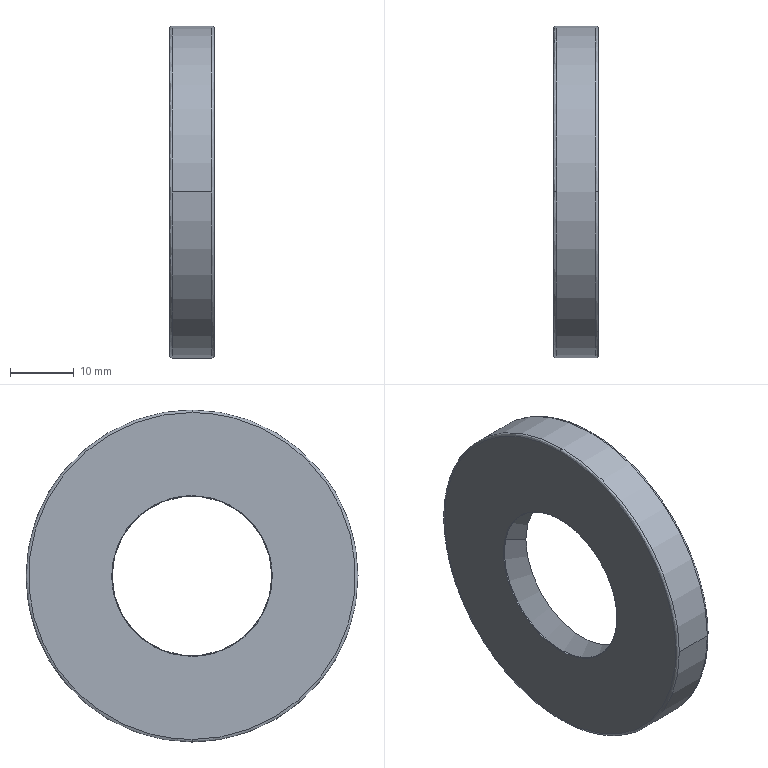Part | SolidWorks | features BaseBody 1 | 1 solid | 30 faces | box 7 x 52 x 52 mm | volume 5117 mm3 | spline 12 | cone 8 | cylinder 6 | plane 4 | commonest cylinder face diameters 32.2 x2 48.5 x2 52 x2